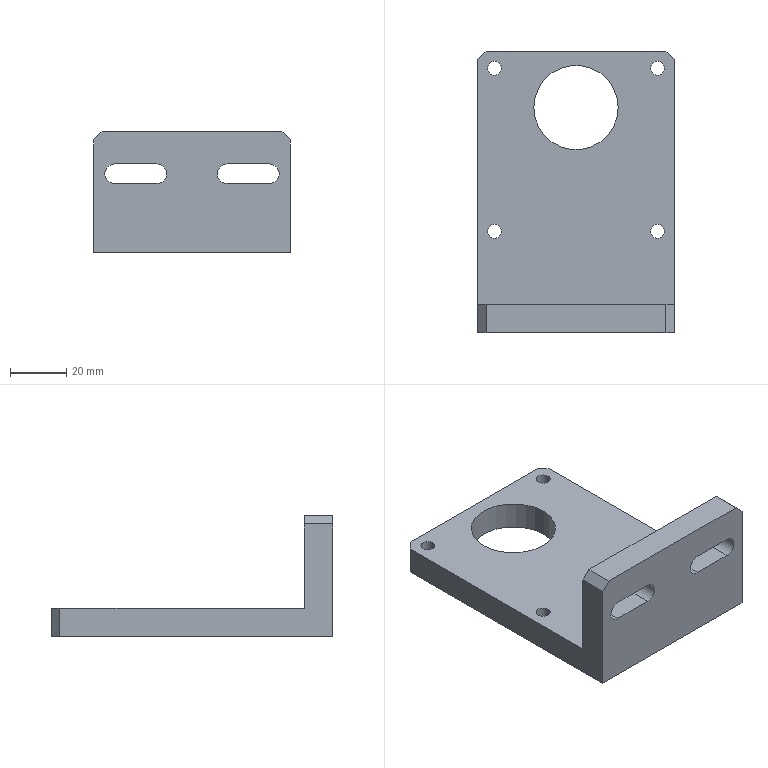Part | STEP file | 10020103U05P11_default | 1 solid | 30 faces | box 70 x 100 x 43 mm | volume 82196 mm3 | plane 16 | cylinder 14 | commonest cylinder face diameters 5 x8 7 x4 30 x2